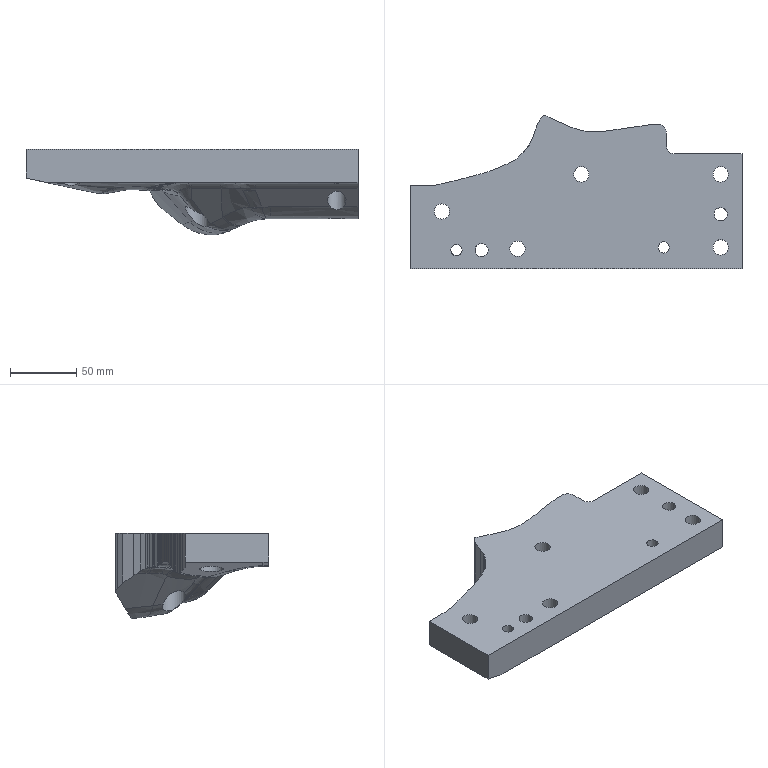Part | STEP file | lll_id826_x_t | 1 solid | 192 faces | box 250 x 115.491 x 64.531 mm | volume 741435 mm3 | spline 84 | plane 77 | cylinder 29 | torus 1 | sphere 1 | commonest cylinder face diameters 11.509 x5 18.008 x5 30 x3 55 x3 8.505 x2 10 x2